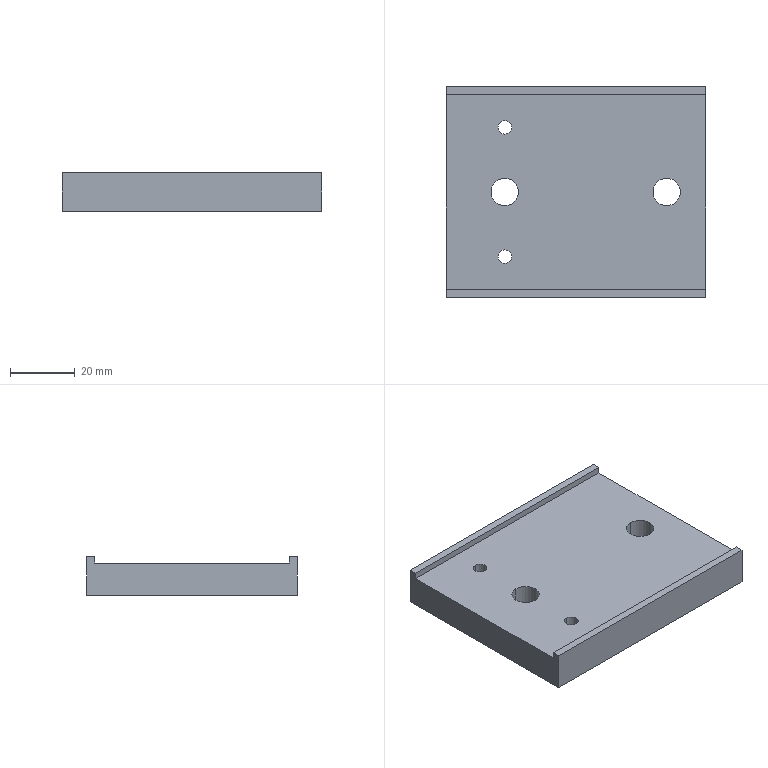CAM job | NX | 3-axis milling, drilling | part box 80 x 65 x 12 mm | stock box 80 x 65 x 12 mm
Tools:
number,name,description,diameter,corner_radius,flute_length,length,flutes
7,D6A45,Milling Tool-5 Parameters,6.0,0.0,3.0,3.0,2
10,D10,Milling Tool-5 Parameters,10.0,0.0,50.0,75.0,2
11,D10JING,Milling Tool-5 Parameters,10.0,0.0,50.0,75.0,2
14,4.2ZT,Drilling Tool,4.2,0.0,35.0,50.0,2
8,8.5ZT,Drilling Tool,8.5,0.0,35.0,50.0,2
Operations:
program,operation,operation_type,tool,method,geometry_group,spindle_rpm,surface_speed,feed_per_tooth,feed_cut,feed_plunge,cut_length_mm,path_length_mm,cut_time_min,machine_time_min
1,FLOOR_WALL,VolumeBased25DMillingOperation,D10,METHOD,A,7500.0,235.0,0.2,3000.0,1000.0,1563.994,1727.491,0.5295,0.5458
1,DRILLING_COPY_1,Operation,D6A45,METHOD,A,3000.0,56.0,0.0333,200.0,0.0,16.0,199.383,0.08,0.0983
1,DRILLING_COPY_1_COPY,Operation,4.2ZT,METHOD,A,2000.0,42.0,0.05,200.0,0.0,31.524,170.16,0.1576,0.1715
1,DRILLING_COPY_1_COPY_COPY,Operation,8.5ZT,METHOD,A,2000.0,42.0,0.05,200.0,0.0,34.107,185.304,0.1705,0.1857
1,FLOOR_WALL_1_COPY_1,VolumeBased25DMillingOperation,D10JING,METHOD,A,7500.0,94.0,0.0733,1100.0,100.0,1047.629,1108.629,0.9524,0.9585
1,ZLEVEL_PROFILE_1_COPY_1_COPY_COPY_1_COPY,ZLevelMilling,D6A45,METHOD,A,7500.0,141.0,0.0667,1000.0,100.0,352.772,578.459,0.3528,0.3753
1,ZLEVEL_PROFILE_1_COPY_1_COPY_COPY_1_COPY_COPY,ZLevelMilling,D6A45,METHOD,A,7500.0,141.0,0.0667,1000.0,100.0,179.672,799.288,0.1797,0.2416
1,刀补11,VolumeBased25DMillingOperation,D10JING,METHOD,A,7500.0,94.0,0.0733,1100.0,100.0,195.208,306.12,0.1775,0.1917